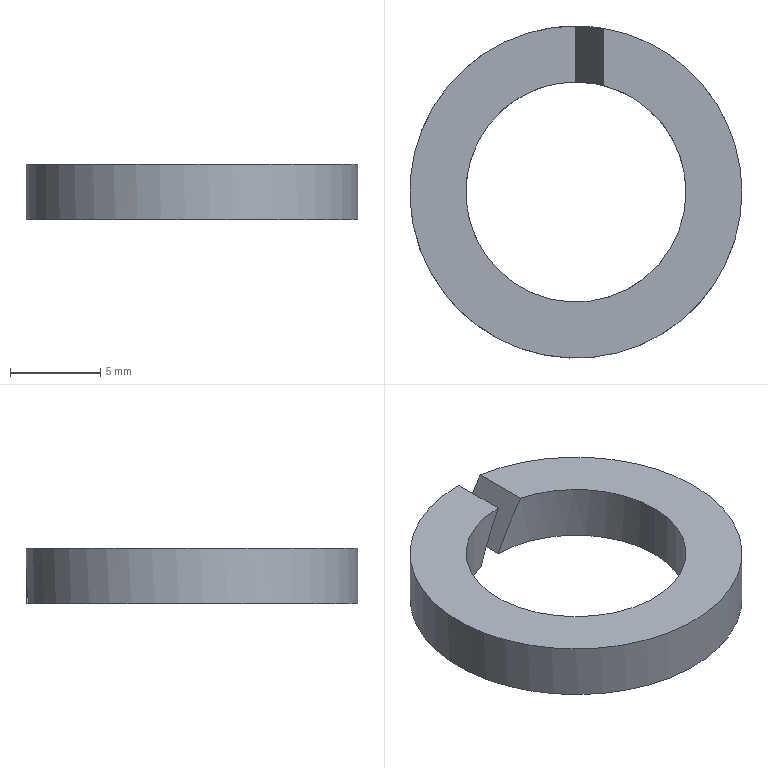Part | NX | features BREP 1 | 1 solid | 8 faces | box 18.4 x 18.4 x 3.1 mm | volume 446.968 mm3 | plane 4 | cylinder 4 | commonest cylinder face diameters 12.2 x2 18.4 x2
STEP:
#1=CARTESIAN_POINT('',(-1.55,5.9,0.));
#2=VERTEX_POINT('',#1);
#3=CARTESIAN_POINT('',(6.1,0.,0.));
#4=VERTEX_POINT('',#3);
#5=CARTESIAN_POINT('',(0.,0.,0.));
#6=DIRECTION('',(0.,0.,1.));
#7=DIRECTION('',(-0.2541,0.9672,0.));
#8=AXIS2_PLACEMENT_3D('',#5,#6,#7);
#9=CIRCLE('',#8,6.1);
#10=EDGE_CURVE('',#2,#4,#9,.T.);
#11=ORIENTED_EDGE('',*,*,#10,.T.);
#12=CARTESIAN_POINT('',(0.,6.1,0.));
#13=VERTEX_POINT('',#12);
#14=CARTESIAN_POINT('',(0.,0.,0.));
#15=DIRECTION('',(0.,0.,-1.));
#16=DIRECTION('',(0.,1.,0.));
#17=AXIS2_PLACEMENT_3D('',#14,#15,#16);
#18=CIRCLE('',#17,6.1);
#19=EDGE_CURVE('',#13,#4,#18,.T.);
#20=ORIENTED_EDGE('',*,*,#19,.F.);
#21=CARTESIAN_POINT('',(0.,9.2,0.));
#22=VERTEX_POINT('',#21);
#23=CARTESIAN_POINT('',(0.,6.1,0.));
#24=DIRECTION('',(0.,1.,0.));
#25=VECTOR('',#24,1000.);
#26=LINE('',#23,#25);
#27=EDGE_CURVE('',#13,#22,#26,.T.);
#28=ORIENTED_EDGE('',*,*,#27,.T.);
#29=CARTESIAN_POINT('',(9.2,0.,0.));
#30=VERTEX_POINT('',#29);
#31=CARTESIAN_POINT('',(0.,0.,0.));
#32=DIRECTION('',(0.,0.,1.));
#33=DIRECTION('',(1.,0.,0.));
#34=AXIS2_PLACEMENT_3D('',#31,#32,#33);
#35=CIRCLE('',#34,9.2);
#36=EDGE_CURVE('',#30,#22,#35,.T.);
#37=ORIENTED_EDGE('',*,*,#36,.F.);
#38=CARTESIAN_POINT('',(-1.55,9.068,0.));
#39=VERTEX_POINT('',#38);
#40=CARTESIAN_POINT('',(0.,0.,0.));
#41=DIRECTION('',(0.,0.,-1.));
#42=DIRECTION('',(1.,0.,0.));
#43=AXIS2_PLACEMENT_3D('',#40,#41,#42);
#44=CIRCLE('',#43,9.2);
#45=EDGE_CURVE('',#30,#39,#44,.T.);
#46=ORIENTED_EDGE('',*,*,#45,.T.);
#47=CARTESIAN_POINT('',(-1.55,5.9,0.));
#48=DIRECTION('',(0.,1.,0.));
#49=VECTOR('',#48,1000.);
#50=LINE('',#47,#49);
#51=EDGE_CURVE('',#2,#39,#50,.T.);
#52=ORIENTED_EDGE('',*,*,#51,.F.);
#53=EDGE_LOOP('',(#11,#20,#28,#37,#46,#52));
#54=FACE_BOUND('',#53,.T.);
#55=CARTESIAN_POINT('',(0.,0.,0.));
#56=DIRECTION('',(0.,0.,1.));
#57=DIRECTION('',(-1.,0.,0.));
#58=AXIS2_PLACEMENT_3D('',#55,#56,#57);
#59=PLANE('',#58);
#60=ADVANCED_FACE('',(#54),#59,.F.);
#61=ORIENTED_EDGE('',*,*,#51,.T.);
#62=CARTESIAN_POINT('',(0.,9.2,3.1));
#63=VERTEX_POINT('',#62);
#64=CARTESIAN_POINT('',(0.,0.,3.1));
#65=DIRECTION('',(-0.8944,0.,0.4472));
#66=DIRECTION('',(0.4472,0.,0.8944));
#67=AXIS2_PLACEMENT_3D('',#64,#65,#66);
#68=ELLIPSE('',#67,20.572,9.2);
#69=EDGE_CURVE('',#63,#39,#68,.T.);
#70=ORIENTED_EDGE('',*,*,#69,.F.);
#71=CARTESIAN_POINT('',(0.,6.1,3.1));
#72=VERTEX_POINT('',#71);
#73=CARTESIAN_POINT('',(0.,6.1,3.1));
#74=DIRECTION('',(0.,1.,0.));
#75=VECTOR('',#74,1000.);
#76=LINE('',#73,#75);
#77=EDGE_CURVE('',#72,#63,#76,.T.);
#78=ORIENTED_EDGE('',*,*,#77,.F.);
#79=CARTESIAN_POINT('',(0.,0.,3.1));
#80=DIRECTION('',(-0.8944,0.,0.4472));
#81=DIRECTION('',(0.4472,0.,0.8944));
#82=AXIS2_PLACEMENT_3D('',#79,#80,#81);
#83=ELLIPSE('',#82,13.64,6.1);
#84=EDGE_CURVE('',#72,#2,#83,.T.);
#85=ORIENTED_EDGE('',*,*,#84,.T.);
#86=EDGE_LOOP('',(#61,#70,#78,#85));
#87=FACE_BOUND('',#86,.T.);
#88=CARTESIAN_POINT('',(-1.55,0.,0.));
#89=DIRECTION('',(-0.8944,0.,0.4472));
#90=DIRECTION('',(-0.4472,0.,-0.8944));
#91=AXIS2_PLACEMENT_3D('',#88,#89,#90);
#92=PLANE('',#91);
#93=ADVANCED_FACE('',(#87),#92,.F.);
#94=CARTESIAN_POINT('',(6.1,0.,3.1));
#95=VERTEX_POINT('',#94);
#96=CARTESIAN_POINT('',(6.1,0.,0.));
#97=DIRECTION('',(0.,0.,1.));
#98=VECTOR('',#97,1000.);
#99=LINE('',#96,#98);
#100=EDGE_CURVE('',#4,#95,#99,.T.);
#101=ORIENTED_EDGE('',*,*,#100,.F.);
#102=ORIENTED_EDGE('',*,*,#10,.F.);
#103=ORIENTED_EDGE('',*,*,#84,.F.);
#104=CARTESIAN_POINT('',(0.,0.,3.1));
#105=DIRECTION('',(0.,0.,-1.));
#106=DIRECTION('',(1.,0.,0.));
#107=AXIS2_PLACEMENT_3D('',#104,#105,#106);
#108=CIRCLE('',#107,6.1);
#109=EDGE_CURVE('',#95,#72,#108,.T.);
#110=ORIENTED_EDGE('',*,*,#109,.F.);
#111=EDGE_LOOP('',(#101,#102,#103,#110));
#112=FACE_BOUND('',#111,.T.);
#113=CARTESIAN_POINT('',(0.,0.,0.));
#114=DIRECTION('',(0.,0.,1.));
#115=DIRECTION('',(-1.,0.,0.));
#116=AXIS2_PLACEMENT_3D('',#113,#114,#115);
#117=CYLINDRICAL_SURFACE('',#116,6.1);
#118=ADVANCED_FACE('',(#112),#117,.F.);
#119=CARTESIAN_POINT('',(9.2,0.,3.1));
#120=VERTEX_POINT('',#119);
#121=CARTESIAN_POINT('',(0.,0.,3.1));
#122=DIRECTION('',(0.,0.,1.));
#123=DIRECTION('',(0.,1.,0.));
#124=AXIS2_PLACEMENT_3D('',#121,#122,#123);
#125=CIRCLE('',#124,9.2);
#126=EDGE_CURVE('',#63,#120,#125,.T.);
#127=ORIENTED_EDGE('',*,*,#126,.T.);
#128=CARTESIAN_POINT('',(1.55,9.068,3.1));
#129=VERTEX_POINT('',#128);
#130=CARTESIAN_POINT('',(0.,0.,3.1));
#131=DIRECTION('',(0.,0.,1.));
#132=DIRECTION('',(1.,0.,0.));
#133=AXIS2_PLACEMENT_3D('',#130,#131,#132);
#134=CIRCLE('',#133,9.2);
#135=EDGE_CURVE('',#120,#129,#134,.T.);
#136=ORIENTED_EDGE('',*,*,#135,.T.);
#137=CARTESIAN_POINT('',(1.55,5.9,3.1));
#138=VERTEX_POINT('',#137);
#139=CARTESIAN_POINT('',(1.55,5.9,3.1));
#140=DIRECTION('',(0.,1.,0.));
#141=VECTOR('',#140,1000.);
#142=LINE('',#139,#141);
#143=EDGE_CURVE('',#138,#129,#142,.T.);
#144=ORIENTED_EDGE('',*,*,#143,.F.);
#145=CARTESIAN_POINT('',(0.,0.,3.1));
#146=DIRECTION('',(0.,0.,-1.));
#147=DIRECTION('',(0.2541,0.9672,0.));
#148=AXIS2_PLACEMENT_3D('',#145,#146,#147);
#149=CIRCLE('',#148,6.1);
#150=EDGE_CURVE('',#138,#95,#149,.T.);
#151=ORIENTED_EDGE('',*,*,#150,.T.);
#152=ORIENTED_EDGE('',*,*,#109,.T.);
#153=ORIENTED_EDGE('',*,*,#77,.T.);
#154=EDGE_LOOP('',(#127,#136,#144,#151,#152,#153));
#155=FACE_BOUND('',#154,.T.);
#156=CARTESIAN_POINT('',(0.,0.,3.1));
#157=DIRECTION('',(0.,0.,1.));
#158=DIRECTION('',(-1.,0.,0.));
#159=AXIS2_PLACEMENT_3D('',#156,#157,#158);
#160=PLANE('',#159);
#161=ADVANCED_FACE('',(#155),#160,.T.);
#162=ORIENTED_EDGE('',*,*,#19,.T.);
#163=ORIENTED_EDGE('',*,*,#100,.T.);
#164=ORIENTED_EDGE('',*,*,#150,.F.);
#165=CARTESIAN_POINT('',(0.,0.,0.));
#166=DIRECTION('',(0.8944,0.,-0.4472));
#167=DIRECTION('',(0.4472,0.,0.8944));
#168=AXIS2_PLACEMENT_3D('',#165,#166,#167);
#169=ELLIPSE('',#168,13.64,6.1);
#170=EDGE_CURVE('',#138,#13,#169,.F.);
#171=ORIENTED_EDGE('',*,*,#170,.T.);
#172=EDGE_LOOP('',(#162,#163,#164,#171));
#173=FACE_BOUND('',#172,.T.);
#174=CARTESIAN_POINT('',(0.,0.,0.));
#175=DIRECTION('',(0.,0.,1.));
#176=DIRECTION('',(-1.,0.,0.));
#177=AXIS2_PLACEMENT_3D('',#174,#175,#176);
#178=CYLINDRICAL_SURFACE('',#177,6.1);
#179=ADVANCED_FACE('',(#173),#178,.F.);
#180=ORIENTED_EDGE('',*,*,#27,.F.);
#181=ORIENTED_EDGE('',*,*,#170,.F.);
#182=ORIENTED_EDGE('',*,*,#143,.T.);
#183=CARTESIAN_POINT('',(0.,0.,0.));
#184=DIRECTION('',(0.8944,0.,-0.4472));
#185=DIRECTION('',(0.4472,0.,0.8944));
#186=AXIS2_PLACEMENT_3D('',#183,#184,#185);
#187=ELLIPSE('',#186,20.572,9.2);
#188=EDGE_CURVE('',#129,#22,#187,.F.);
#189=ORIENTED_EDGE('',*,*,#188,.T.);
#190=EDGE_LOOP('',(#180,#181,#182,#189));
#191=FACE_BOUND('',#190,.T.);
#192=CARTESIAN_POINT('',(1.55,0.,3.1));
#193=DIRECTION('',(0.8944,0.,-0.4472));
#194=DIRECTION('',(0.4472,0.,0.8944));
#195=AXIS2_PLACEMENT_3D('',#192,#193,#194);
#196=PLANE('',#195);
#197=ADVANCED_FACE('',(#191),#196,.F.);
#198=ORIENTED_EDGE('',*,*,#135,.F.);
#199=CARTESIAN_POINT('',(9.2,0.,0.));
#200=DIRECTION('',(0.,0.,1.));
#201=VECTOR('',#200,1000.);
#202=LINE('',#199,#201);
#203=EDGE_CURVE('',#30,#120,#202,.T.);
#204=ORIENTED_EDGE('',*,*,#203,.F.);
#205=ORIENTED_EDGE('',*,*,#36,.T.);
#206=ORIENTED_EDGE('',*,*,#188,.F.);
#207=EDGE_LOOP('',(#198,#204,#205,#206));
#208=FACE_BOUND('',#207,.T.);
#209=CARTESIAN_POINT('',(0.,0.,0.));
#210=DIRECTION('',(0.,0.,1.));
#211=DIRECTION('',(-1.,0.,0.));
#212=AXIS2_PLACEMENT_3D('',#209,#210,#211);
#213=CYLINDRICAL_SURFACE('',#212,9.2);
#214=ADVANCED_FACE('',(#208),#213,.T.);
#215=ORIENTED_EDGE('',*,*,#203,.T.);
#216=ORIENTED_EDGE('',*,*,#126,.F.);
#217=ORIENTED_EDGE('',*,*,#69,.T.);
#218=ORIENTED_EDGE('',*,*,#45,.F.);
#219=EDGE_LOOP('',(#215,#216,#217,#218));
#220=FACE_BOUND('',#219,.T.);
#221=CARTESIAN_POINT('',(0.,0.,0.));
#222=DIRECTION('',(0.,0.,1.));
#223=DIRECTION('',(-1.,0.,0.));
#224=AXIS2_PLACEMENT_3D('',#221,#222,#223);
#225=CYLINDRICAL_SURFACE('',#224,9.2);
#226=ADVANCED_FACE('',(#220),#225,.T.);
#227=CLOSED_SHELL('',(#60,#93,#118,#161,#179,#197,#214,#226));
#228=MANIFOLD_SOLID_BREP('',#227);
#229=(LENGTH_UNIT()NAMED_UNIT(*)SI_UNIT(.MILLI.,.METRE.));
#230=UNCERTAINTY_MEASURE_WITH_UNIT(LENGTH_MEASURE(0.00001),#229,'','');
#231=(NAMED_UNIT(*)PLANE_ANGLE_UNIT()SI_UNIT($,.RADIAN.));
#232=(NAMED_UNIT(*)SI_UNIT($,.STERADIAN.)SOLID_ANGLE_UNIT());
#233=(GEOMETRIC_REPRESENTATION_CONTEXT(3)GLOBAL_UNCERTAINTY_ASSIGNED_CONTEXT((#230))GLOBAL_UNIT_ASSIGNED_CONTEXT((#229,#231,#232))REPRESENTATION_CONTEXT('',''));
#234=ADVANCED_BREP_SHAPE_REPRESENTATION('',(#228),#233);